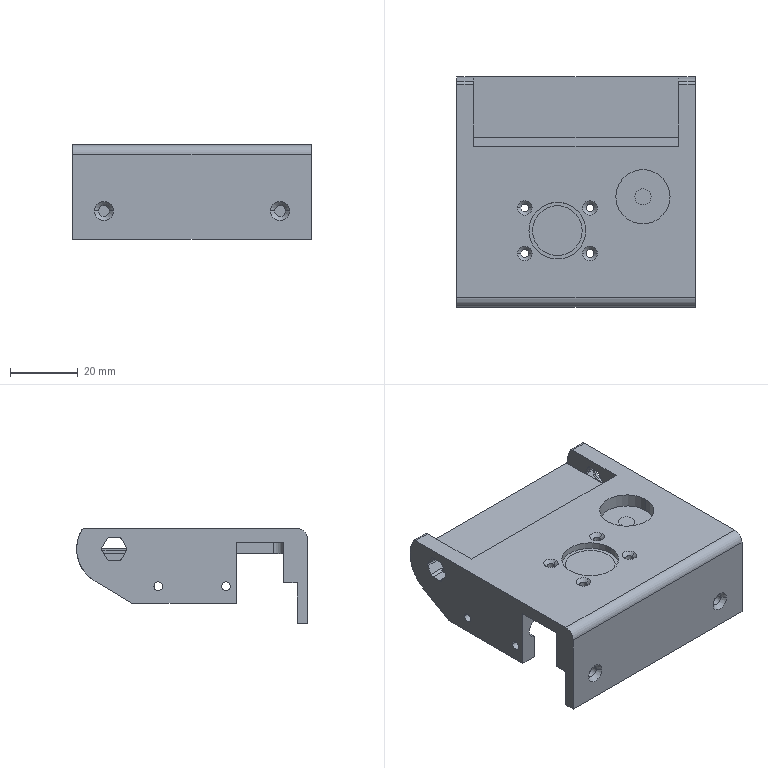NC program | NX | posted with a generic post | part box 70.5 x 68.1 x 28 mm
Whole program:
N10 G17 G21 G94 G90
(DRILLING_1 , TOOL : D6A45)
N12 T07 M6
N14 G54
N16 G17 G0 G90 X-26. Y-19.6 B0. C0. S3500 M3
N18 G43 Z30. H7
N20 G94 G81 G98 Z-2.8 F250. R3.
N22 X26.
N24 G80
N26 G0 X26. Y-19.6 Z30.
N28 M5
(DRILLING_COPY_COPY_1 , TOOL : 3.2ZT)
N30 T13 M6
N32 G54
N34 G17 G0 G90 X-26. Y-19.6 B0. C0. S2500 M3
N36 G43 Z30. H13
N38 G94 G83 G98 Z-5.461 F120. Q2. R3.
N40 X26.
N42 G80
N44 G0 X26. Y-19.6 Z30.
N46 M5
N48 M2